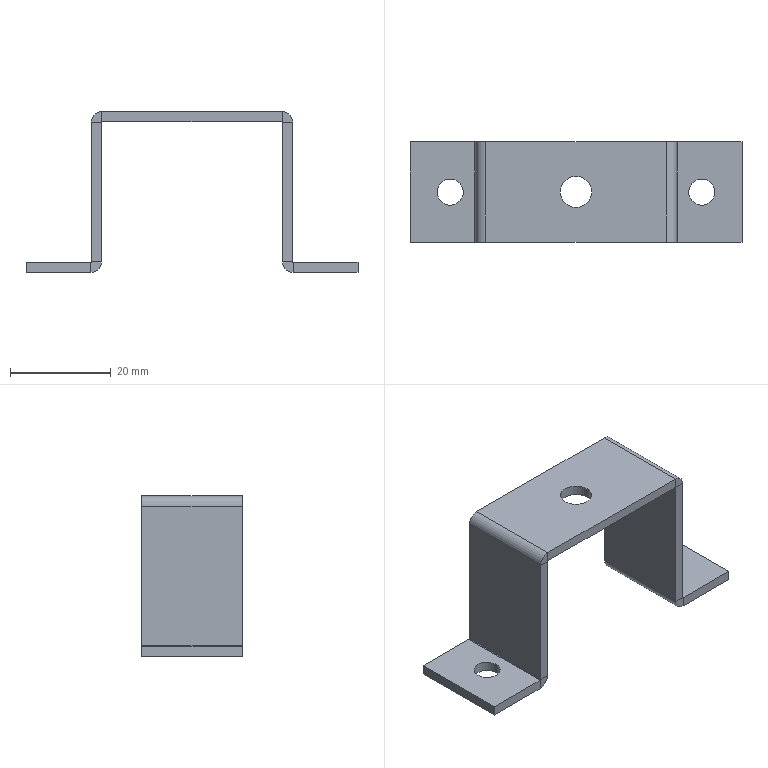Part | SolidWorks | features EdgeFlange 2, FlatPattern 1, HoleWzd 1, ICE 1, SMBaseFlange 1, SheetMetal 1 | 1 solid | 44 faces | box 66 x 20 x 32 mm | volume 4819 mm3 | plane 30 | cylinder 14 | commonest cylinder face diameters 0.2 x4 4.2 x4 5.2 x4 6.2 x2
STEP:
#1=CARTESIAN_POINT('',(-27.6,0.,-32.));
#2=VERTEX_POINT('',#1);
#3=CARTESIAN_POINT('',(-22.4,0.,-32.));
#4=VERTEX_POINT('',#3);
#5=CARTESIAN_POINT('',(-25.,0.,-32.));
#6=DIRECTION('',(0.,0.,1.));
#7=DIRECTION('',(1.,0.,0.));
#8=AXIS2_PLACEMENT_3D('',#5,#6,#7);
#9=CIRCLE('',#8,2.6);
#10=EDGE_CURVE('',#2,#4,#9,.T.);
#11=ORIENTED_EDGE('',*,*,#10,.F.);
#12=CARTESIAN_POINT('',(-27.6,0.,-30.));
#13=VERTEX_POINT('',#12);
#14=CARTESIAN_POINT('',(-27.6,0.,-30.));
#15=DIRECTION('',(0.,0.,1.));
#16=VECTOR('',#15,1000.);
#17=LINE('',#14,#16);
#18=EDGE_CURVE('',#2,#13,#17,.T.);
#19=ORIENTED_EDGE('',*,*,#18,.T.);
#20=CARTESIAN_POINT('',(-22.4,0.,-30.));
#21=VERTEX_POINT('',#20);
#22=CARTESIAN_POINT('',(-25.,0.,-30.));
#23=DIRECTION('',(0.,0.,1.));
#24=DIRECTION('',(1.,0.,0.));
#25=AXIS2_PLACEMENT_3D('',#22,#23,#24);
#26=CIRCLE('',#25,2.6);
#27=EDGE_CURVE('',#13,#21,#26,.T.);
#28=ORIENTED_EDGE('',*,*,#27,.T.);
#29=CARTESIAN_POINT('',(-22.4,0.,-30.));
#30=DIRECTION('',(0.,0.,1.));
#31=VECTOR('',#30,1000.);
#32=LINE('',#29,#31);
#33=EDGE_CURVE('',#4,#21,#32,.T.);
#34=ORIENTED_EDGE('',*,*,#33,.F.);
#35=EDGE_LOOP('',(#11,#19,#28,#34));
#36=FACE_OUTER_BOUND('',#35,.T.);
#37=CARTESIAN_POINT('',(-25.,0.,-30.));
#38=DIRECTION('',(0.,0.,1.));
#39=DIRECTION('',(1.,0.,0.));
#40=AXIS2_PLACEMENT_3D('',#37,#38,#39);
#41=CYLINDRICAL_SURFACE('',#40,2.6);
#42=ADVANCED_FACE('',(#36),#41,.F.);
#43=CARTESIAN_POINT('',(22.4,0.,-32.));
#44=VERTEX_POINT('',#43);
#45=CARTESIAN_POINT('',(27.6,0.,-32.));
#46=VERTEX_POINT('',#45);
#47=CARTESIAN_POINT('',(25.,0.,-32.));
#48=DIRECTION('',(0.,0.,1.));
#49=DIRECTION('',(1.,0.,0.));
#50=AXIS2_PLACEMENT_3D('',#47,#48,#49);
#51=CIRCLE('',#50,2.6);
#52=EDGE_CURVE('',#44,#46,#51,.T.);
#53=ORIENTED_EDGE('',*,*,#52,.F.);
#54=CARTESIAN_POINT('',(22.4,0.,-30.));
#55=VERTEX_POINT('',#54);
#56=CARTESIAN_POINT('',(22.4,0.,-30.));
#57=DIRECTION('',(0.,0.,1.));
#58=VECTOR('',#57,1000.);
#59=LINE('',#56,#58);
#60=EDGE_CURVE('',#44,#55,#59,.T.);
#61=ORIENTED_EDGE('',*,*,#60,.T.);
#62=CARTESIAN_POINT('',(27.6,0.,-30.));
#63=VERTEX_POINT('',#62);
#64=CARTESIAN_POINT('',(25.,0.,-30.));
#65=DIRECTION('',(0.,0.,1.));
#66=DIRECTION('',(1.,0.,0.));
#67=AXIS2_PLACEMENT_3D('',#64,#65,#66);
#68=CIRCLE('',#67,2.6);
#69=EDGE_CURVE('',#55,#63,#68,.T.);
#70=ORIENTED_EDGE('',*,*,#69,.T.);
#71=CARTESIAN_POINT('',(27.6,0.,-30.));
#72=DIRECTION('',(0.,0.,1.));
#73=VECTOR('',#72,1000.);
#74=LINE('',#71,#73);
#75=EDGE_CURVE('',#46,#63,#74,.T.);
#76=ORIENTED_EDGE('',*,*,#75,.F.);
#77=EDGE_LOOP('',(#53,#61,#70,#76));
#78=FACE_OUTER_BOUND('',#77,.T.);
#79=CARTESIAN_POINT('',(25.,0.,-30.));
#80=DIRECTION('',(0.,0.,1.));
#81=DIRECTION('',(1.,0.,0.));
#82=AXIS2_PLACEMENT_3D('',#79,#80,#81);
#83=CYLINDRICAL_SURFACE('',#82,2.6);
#84=ADVANCED_FACE('',(#78),#83,.F.);
#85=CARTESIAN_POINT('',(3.1,0.,-2.));
#86=VERTEX_POINT('',#85);
#87=CARTESIAN_POINT('',(-3.1,0.,-2.));
#88=VERTEX_POINT('',#87);
#89=CARTESIAN_POINT('',(0.,0.,-2.));
#90=DIRECTION('',(0.,0.,-1.));
#91=DIRECTION('',(1.,0.,0.));
#92=AXIS2_PLACEMENT_3D('',#89,#90,#91);
#93=CIRCLE('',#92,3.1);
#94=EDGE_CURVE('',#86,#88,#93,.T.);
#95=ORIENTED_EDGE('',*,*,#94,.T.);
#96=CARTESIAN_POINT('',(-3.1,0.,0.));
#97=VERTEX_POINT('',#96);
#98=CARTESIAN_POINT('',(-3.1,0.,-32.001));
#99=DIRECTION('',(0.,0.,1.));
#100=VECTOR('',#99,1000.);
#101=LINE('',#98,#100);
#102=EDGE_CURVE('',#88,#97,#101,.T.);
#103=ORIENTED_EDGE('',*,*,#102,.T.);
#104=CARTESIAN_POINT('',(3.1,0.,0.));
#105=VERTEX_POINT('',#104);
#106=CARTESIAN_POINT('',(0.,0.,0.));
#107=DIRECTION('',(0.,0.,1.));
#108=DIRECTION('',(1.,0.,0.));
#109=AXIS2_PLACEMENT_3D('',#106,#107,#108);
#110=CIRCLE('',#109,3.1);
#111=EDGE_CURVE('',#97,#105,#110,.T.);
#112=ORIENTED_EDGE('',*,*,#111,.T.);
#113=CARTESIAN_POINT('',(3.1,0.,-32.001));
#114=DIRECTION('',(0.,0.,1.));
#115=VECTOR('',#114,1000.);
#116=LINE('',#113,#115);
#117=EDGE_CURVE('',#86,#105,#116,.T.);
#118=ORIENTED_EDGE('',*,*,#117,.F.);
#119=EDGE_LOOP('',(#95,#103,#112,#118));
#120=FACE_OUTER_BOUND('',#119,.T.);
#121=CARTESIAN_POINT('',(0.,0.,-32.001));
#122=DIRECTION('',(0.,0.,1.));
#123=DIRECTION('',(1.,0.,0.));
#124=AXIS2_PLACEMENT_3D('',#121,#122,#123);
#125=CYLINDRICAL_SURFACE('',#124,3.1);
#126=ADVANCED_FACE('',(#120),#125,.F.);
#127=CARTESIAN_POINT('',(20.,10.,-2.1));
#128=VERTEX_POINT('',#127);
#129=CARTESIAN_POINT('',(20.,10.,-29.9));
#130=VERTEX_POINT('',#129);
#131=CARTESIAN_POINT('',(20.,10.,-2.));
#132=DIRECTION('',(0.,0.,-1.));
#133=VECTOR('',#132,1000.);
#134=LINE('',#131,#133);
#135=EDGE_CURVE('',#128,#130,#134,.T.);
#136=ORIENTED_EDGE('',*,*,#135,.T.);
#137=CARTESIAN_POINT('',(18.,10.,-29.9));
#138=VERTEX_POINT('',#137);
#139=CARTESIAN_POINT('',(20.,10.,-29.9));
#140=DIRECTION('',(-1.,0.,0.));
#141=VECTOR('',#140,1000.);
#142=LINE('',#139,#141);
#143=EDGE_CURVE('',#130,#138,#142,.T.);
#144=ORIENTED_EDGE('',*,*,#143,.T.);
#145=CARTESIAN_POINT('',(18.,10.,-2.1));
#146=VERTEX_POINT('',#145);
#147=CARTESIAN_POINT('',(18.,10.,0.));
#148=DIRECTION('',(0.,0.,-1.));
#149=VECTOR('',#148,1000.);
#150=LINE('',#147,#149);
#151=EDGE_CURVE('',#146,#138,#150,.T.);
#152=ORIENTED_EDGE('',*,*,#151,.F.);
#153=CARTESIAN_POINT('',(20.,10.,-2.1));
#154=DIRECTION('',(1.,0.,0.));
#155=VECTOR('',#154,1000.);
#156=LINE('',#153,#155);
#157=EDGE_CURVE('',#146,#128,#156,.T.);
#158=ORIENTED_EDGE('',*,*,#157,.T.);
#159=EDGE_LOOP('',(#136,#144,#152,#158));
#160=FACE_OUTER_BOUND('',#159,.T.);
#161=CARTESIAN_POINT('',(20.,10.,-2.));
#162=DIRECTION('',(0.,1.,0.));
#163=DIRECTION('',(0.,0.,1.));
#164=AXIS2_PLACEMENT_3D('',#161,#162,#163);
#165=PLANE('',#164);
#166=ADVANCED_FACE('',(#160),#165,.T.);
#167=CARTESIAN_POINT('',(20.,-10.,-29.9));
#168=VERTEX_POINT('',#167);
#169=CARTESIAN_POINT('',(20.,10.,-29.9));
#170=DIRECTION('',(0.,-1.,0.));
#171=VECTOR('',#170,1000.);
#172=LINE('',#169,#171);
#173=EDGE_CURVE('',#130,#168,#172,.T.);
#174=ORIENTED_EDGE('',*,*,#173,.F.);
#175=ORIENTED_EDGE('',*,*,#135,.F.);
#176=CARTESIAN_POINT('',(20.,-10.,-2.1));
#177=VERTEX_POINT('',#176);
#178=CARTESIAN_POINT('',(20.,10.,-2.1));
#179=DIRECTION('',(0.,1.,0.));
#180=VECTOR('',#179,1000.);
#181=LINE('',#178,#180);
#182=EDGE_CURVE('',#177,#128,#181,.T.);
#183=ORIENTED_EDGE('',*,*,#182,.F.);
#184=CARTESIAN_POINT('',(20.,-10.,-32.));
#185=DIRECTION('',(0.,0.,1.));
#186=VECTOR('',#185,1000.);
#187=LINE('',#184,#186);
#188=EDGE_CURVE('',#168,#177,#187,.T.);
#189=ORIENTED_EDGE('',*,*,#188,.F.);
#190=EDGE_LOOP('',(#174,#175,#183,#189));
#191=FACE_OUTER_BOUND('',#190,.T.);
#192=CARTESIAN_POINT('',(20.,0.,0.));
#193=DIRECTION('',(-1.,0.,0.));
#194=DIRECTION('',(0.,0.,1.));
#195=AXIS2_PLACEMENT_3D('',#192,#193,#194);
#196=PLANE('',#195);
#197=ADVANCED_FACE('',(#191),#196,.F.);
#198=ORIENTED_EDGE('',*,*,#151,.T.);
#199=CARTESIAN_POINT('',(18.,-10.,-29.9));
#200=VERTEX_POINT('',#199);
#201=CARTESIAN_POINT('',(18.,10.,-29.9));
#202=DIRECTION('',(0.,-1.,0.));
#203=VECTOR('',#202,1000.);
#204=LINE('',#201,#203);
#205=EDGE_CURVE('',#138,#200,#204,.T.);
#206=ORIENTED_EDGE('',*,*,#205,.T.);
#207=CARTESIAN_POINT('',(18.,-10.,-2.1));
#208=VERTEX_POINT('',#207);
#209=CARTESIAN_POINT('',(18.,-10.,0.));
#210=DIRECTION('',(0.,0.,1.));
#211=VECTOR('',#210,1000.);
#212=LINE('',#209,#211);
#213=EDGE_CURVE('',#200,#208,#212,.T.);
#214=ORIENTED_EDGE('',*,*,#213,.T.);
#215=CARTESIAN_POINT('',(18.,10.,-2.1));
#216=DIRECTION('',(0.,-1.,0.));
#217=VECTOR('',#216,1000.);
#218=LINE('',#215,#217);
#219=EDGE_CURVE('',#146,#208,#218,.T.);
#220=ORIENTED_EDGE('',*,*,#219,.F.);
#221=EDGE_LOOP('',(#198,#206,#214,#220));
#222=FACE_OUTER_BOUND('',#221,.T.);
#223=CARTESIAN_POINT('',(18.,0.,0.));
#224=DIRECTION('',(-1.,0.,0.));
#225=DIRECTION('',(0.,0.,1.));
#226=AXIS2_PLACEMENT_3D('',#223,#224,#225);
#227=PLANE('',#226);
#228=ADVANCED_FACE('',(#222),#227,.T.);
#229=CARTESIAN_POINT('',(-20.,-10.,-2.1));
#230=VERTEX_POINT('',#229);
#231=CARTESIAN_POINT('',(-20.,-10.,-29.9));
#232=VERTEX_POINT('',#231);
#233=CARTESIAN_POINT('',(-20.,-10.,-32.));
#234=DIRECTION('',(0.,0.,-1.));
#235=VECTOR('',#234,1000.);
#236=LINE('',#233,#235);
#237=EDGE_CURVE('',#230,#232,#236,.T.);
#238=ORIENTED_EDGE('',*,*,#237,.T.);
#239=CARTESIAN_POINT('',(-18.,-10.,-29.9));
#240=VERTEX_POINT('',#239);
#241=CARTESIAN_POINT('',(-20.,-10.,-29.9));
#242=DIRECTION('',(1.,0.,0.));
#243=VECTOR('',#242,1000.);
#244=LINE('',#241,#243);
#245=EDGE_CURVE('',#232,#240,#244,.T.);
#246=ORIENTED_EDGE('',*,*,#245,.T.);
#247=CARTESIAN_POINT('',(-18.,-10.,-2.1));
#248=VERTEX_POINT('',#247);
#249=CARTESIAN_POINT('',(-18.,-10.,0.));
#250=DIRECTION('',(0.,0.,-1.));
#251=VECTOR('',#250,1000.);
#252=LINE('',#249,#251);
#253=EDGE_CURVE('',#248,#240,#252,.T.);
#254=ORIENTED_EDGE('',*,*,#253,.F.);
#255=CARTESIAN_POINT('',(-20.,-10.,-2.1));
#256=DIRECTION('',(-1.,0.,0.));
#257=VECTOR('',#256,1000.);
#258=LINE('',#255,#257);
#259=EDGE_CURVE('',#248,#230,#258,.T.);
#260=ORIENTED_EDGE('',*,*,#259,.T.);
#261=EDGE_LOOP('',(#238,#246,#254,#260));
#262=FACE_OUTER_BOUND('',#261,.T.);
#263=CARTESIAN_POINT('',(-20.,-10.,-32.));
#264=DIRECTION('',(0.,-1.,0.));
#265=DIRECTION('',(0.,0.,-1.));
#266=AXIS2_PLACEMENT_3D('',#263,#264,#265);
#267=PLANE('',#266);
#268=ADVANCED_FACE('',(#262),#267,.T.);
#269=CARTESIAN_POINT('',(-20.,10.,-29.9));
#270=VERTEX_POINT('',#269);
#271=CARTESIAN_POINT('',(-20.,10.,-2.1));
#272=VERTEX_POINT('',#271);
#273=CARTESIAN_POINT('',(-20.,10.,-2.));
#274=DIRECTION('',(0.,0.,1.));
#275=VECTOR('',#274,1000.);
#276=LINE('',#273,#275);
#277=EDGE_CURVE('',#270,#272,#276,.T.);
#278=ORIENTED_EDGE('',*,*,#277,.F.);
#279=CARTESIAN_POINT('',(-20.,-10.,-29.9));
#280=DIRECTION('',(0.,1.,0.));
#281=VECTOR('',#280,1000.);
#282=LINE('',#279,#281);
#283=EDGE_CURVE('',#232,#270,#282,.T.);
#284=ORIENTED_EDGE('',*,*,#283,.F.);
#285=ORIENTED_EDGE('',*,*,#237,.F.);
#286=CARTESIAN_POINT('',(-20.,0.,-2.1));
#287=DIRECTION('',(0.,1.,0.));
#288=VECTOR('',#287,1000.);
#289=LINE('',#286,#288);
#290=EDGE_CURVE('',#230,#272,#289,.T.);
#291=ORIENTED_EDGE('',*,*,#290,.T.);
#292=EDGE_LOOP('',(#278,#284,#285,#291));
#293=FACE_OUTER_BOUND('',#292,.T.);
#294=CARTESIAN_POINT('',(-20.,0.,0.));
#295=DIRECTION('',(-1.,0.,0.));
#296=DIRECTION('',(0.,0.,1.));
#297=AXIS2_PLACEMENT_3D('',#294,#295,#296);
#298=PLANE('',#297);
#299=ADVANCED_FACE('',(#293),#298,.T.);
#300=CARTESIAN_POINT('',(-18.,10.,-29.9));
#301=VERTEX_POINT('',#300);
#302=CARTESIAN_POINT('',(-18.,-10.,-29.9));
#303=DIRECTION('',(0.,1.,0.));
#304=VECTOR('',#303,1000.);
#305=LINE('',#302,#304);
#306=EDGE_CURVE('',#240,#301,#305,.T.);
#307=ORIENTED_EDGE('',*,*,#306,.T.);
#308=CARTESIAN_POINT('',(-18.,10.,-2.1));
#309=VERTEX_POINT('',#308);
#310=CARTESIAN_POINT('',(-18.,10.,0.));
#311=DIRECTION('',(0.,0.,1.));
#312=VECTOR('',#311,1000.);
#313=LINE('',#310,#312);
#314=EDGE_CURVE('',#301,#309,#313,.T.);
#315=ORIENTED_EDGE('',*,*,#314,.T.);
#316=CARTESIAN_POINT('',(-18.,-10.,-2.1));
#317=DIRECTION('',(0.,1.,0.));
#318=VECTOR('',#317,1000.);
#319=LINE('',#316,#318);
#320=EDGE_CURVE('',#248,#309,#319,.T.);
#321=ORIENTED_EDGE('',*,*,#320,.F.);
#322=ORIENTED_EDGE('',*,*,#253,.T.);
#323=EDGE_LOOP('',(#307,#315,#321,#322));
#324=FACE_OUTER_BOUND('',#323,.T.);
#325=CARTESIAN_POINT('',(-18.,0.,0.));
#326=DIRECTION('',(-1.,0.,0.));
#327=DIRECTION('',(0.,0.,1.));
#328=AXIS2_PLACEMENT_3D('',#325,#326,#327);
#329=PLANE('',#328);
#330=ADVANCED_FACE('',(#324),#329,.F.);
#331=ORIENTED_EDGE('',*,*,#94,.F.);
#332=CARTESIAN_POINT('',(0.,0.,-2.));
#333=DIRECTION('',(0.,0.,-1.));
#334=DIRECTION('',(1.,0.,0.));
#335=AXIS2_PLACEMENT_3D('',#332,#333,#334);
#336=CIRCLE('',#335,3.1);
#337=EDGE_CURVE('',#88,#86,#336,.T.);
#338=ORIENTED_EDGE('',*,*,#337,.F.);
#339=EDGE_LOOP('',(#331,#338));
#340=FACE_BOUND('',#339,.T.);
#341=CARTESIAN_POINT('',(17.9,-10.,-2.));
#342=VERTEX_POINT('',#341);
#343=CARTESIAN_POINT('',(17.9,10.,-2.));
#344=VERTEX_POINT('',#343);
#345=CARTESIAN_POINT('',(17.9,-10.,-2.));
#346=DIRECTION('',(0.,1.,0.));
#347=VECTOR('',#346,1000.);
#348=LINE('',#345,#347);
#349=EDGE_CURVE('',#342,#344,#348,.T.);
#350=ORIENTED_EDGE('',*,*,#349,.F.);
#351=CARTESIAN_POINT('',(-17.9,-10.,-2.));
#352=VERTEX_POINT('',#351);
#353=CARTESIAN_POINT('',(-20.,-10.,-2.));
#354=DIRECTION('',(1.,0.,0.));
#355=VECTOR('',#354,1000.);
#356=LINE('',#353,#355);
#357=EDGE_CURVE('',#352,#342,#356,.T.);
#358=ORIENTED_EDGE('',*,*,#357,.F.);
#359=CARTESIAN_POINT('',(-17.9,10.,-2.));
#360=VERTEX_POINT('',#359);
#361=CARTESIAN_POINT('',(-17.9,10.,-2.));
#362=DIRECTION('',(0.,-1.,0.));
#363=VECTOR('',#362,1000.);
#364=LINE('',#361,#363);
#365=EDGE_CURVE('',#360,#352,#364,.T.);
#366=ORIENTED_EDGE('',*,*,#365,.F.);
#367=CARTESIAN_POINT('',(-20.,10.,-2.));
#368=DIRECTION('',(-1.,0.,0.));
#369=VECTOR('',#368,1000.);
#370=LINE('',#367,#369);
#371=EDGE_CURVE('',#344,#360,#370,.T.);
#372=ORIENTED_EDGE('',*,*,#371,.F.);
#373=EDGE_LOOP('',(#350,#358,#366,#372));
#374=FACE_OUTER_BOUND('',#373,.T.);
#375=CARTESIAN_POINT('',(0.,0.,-2.));
#376=DIRECTION('',(0.,0.,1.));
#377=DIRECTION('',(1.,0.,0.));
#378=AXIS2_PLACEMENT_3D('',#375,#376,#377);
#379=PLANE('',#378);
#380=ADVANCED_FACE('',(#340,#374),#379,.F.);
#381=CARTESIAN_POINT('',(0.,0.,0.));
#382=DIRECTION('',(0.,0.,1.));
#383=DIRECTION('',(1.,0.,0.));
#384=AXIS2_PLACEMENT_3D('',#381,#382,#383);
#385=CIRCLE('',#384,3.1);
#386=EDGE_CURVE('',#105,#97,#385,.T.);
#387=ORIENTED_EDGE('',*,*,#386,.F.);
#388=ORIENTED_EDGE('',*,*,#111,.F.);
#389=EDGE_LOOP('',(#387,#388));
#390=FACE_BOUND('',#389,.T.);
#391=CARTESIAN_POINT('',(-17.9,-10.,0.));
#392=VERTEX_POINT('',#391);
#393=CARTESIAN_POINT('',(17.9,-10.,0.));
#394=VERTEX_POINT('',#393);
#395=CARTESIAN_POINT('',(-20.,-10.,0.));
#396=DIRECTION('',(1.,0.,0.));
#397=VECTOR('',#396,1000.);
#398=LINE('',#395,#397);
#399=EDGE_CURVE('',#392,#394,#398,.T.);
#400=ORIENTED_EDGE('',*,*,#399,.T.);
#401=CARTESIAN_POINT('',(17.9,10.,0.));
#402=VERTEX_POINT('',#401);
#403=CARTESIAN_POINT('',(17.9,-10.,0.));
#404=DIRECTION('',(0.,1.,0.));
#405=VECTOR('',#404,1000.);
#406=LINE('',#403,#405);
#407=EDGE_CURVE('',#394,#402,#406,.T.);
#408=ORIENTED_EDGE('',*,*,#407,.T.);
#409=CARTESIAN_POINT('',(-17.9,10.,0.));
#410=VERTEX_POINT('',#409);
#411=CARTESIAN_POINT('',(-20.,10.,0.));
#412=DIRECTION('',(-1.,0.,0.));
#413=VECTOR('',#412,1000.);
#414=LINE('',#411,#413);
#415=EDGE_CURVE('',#402,#410,#414,.T.);
#416=ORIENTED_EDGE('',*,*,#415,.T.);
#417=CARTESIAN_POINT('',(-17.9,10.,0.));
#418=DIRECTION('',(0.,-1.,0.));
#419=VECTOR('',#418,1000.);
#420=LINE('',#417,#419);
#421=EDGE_CURVE('',#410,#392,#420,.T.);
#422=ORIENTED_EDGE('',*,*,#421,.T.);
#423=EDGE_LOOP('',(#400,#408,#416,#422));
#424=FACE_OUTER_BOUND('',#423,.T.);
#425=CARTESIAN_POINT('',(0.,0.,0.));
#426=DIRECTION('',(0.,0.,1.));
#427=DIRECTION('',(1.,0.,0.));
#428=AXIS2_PLACEMENT_3D('',#425,#426,#427);
#429=PLANE('',#428);
#430=ADVANCED_FACE('',(#390,#424),#429,.T.);
#431=ORIENTED_EDGE('',*,*,#357,.T.);
#432=CARTESIAN_POINT('',(17.9,-10.,-2.));
#433=DIRECTION('',(0.,0.,1.));
#434=VECTOR('',#433,1000.);
#435=LINE('',#432,#434);
#436=EDGE_CURVE('',#342,#394,#435,.T.);
#437=ORIENTED_EDGE('',*,*,#436,.T.);
#438=ORIENTED_EDGE('',*,*,#399,.F.);
#439=CARTESIAN_POINT('',(-17.9,-10.,-2.));
#440=DIRECTION('',(0.,0.,1.));
#441=VECTOR('',#440,1000.);
#442=LINE('',#439,#441);
#443=EDGE_CURVE('',#352,#392,#442,.T.);
#444=ORIENTED_EDGE('',*,*,#443,.F.);
#445=EDGE_LOOP('',(#431,#437,#438,#444));
#446=FACE_OUTER_BOUND('',#445,.T.);
#447=CARTESIAN_POINT('',(-20.,-10.,-2.));
#448=DIRECTION('',(0.,-1.,0.));
#449=DIRECTION('',(0.,0.,-1.));
#450=AXIS2_PLACEMENT_3D('',#447,#448,#449);
#451=PLANE('',#450);
#452=ADVANCED_FACE('',(#446),#451,.T.);
#453=CARTESIAN_POINT('',(17.9,10.,-2.));
#454=DIRECTION('',(0.,0.,1.));
#455=VECTOR('',#454,1000.);
#456=LINE('',#453,#455);
#457=EDGE_CURVE('',#344,#402,#456,.T.);
#458=ORIENTED_EDGE('',*,*,#457,.F.);
#459=ORIENTED_EDGE('',*,*,#371,.T.);
#460=CARTESIAN_POINT('',(-17.9,10.,-2.));
#461=DIRECTION('',(0.,0.,1.));
#462=VECTOR('',#461,1000.);
#463=LINE('',#460,#462);
#464=EDGE_CURVE('',#360,#410,#463,.T.);
#465=ORIENTED_EDGE('',*,*,#464,.T.);
#466=ORIENTED_EDGE('',*,*,#415,.F.);
#467=EDGE_LOOP('',(#458,#459,#465,#466));
#468=FACE_OUTER_BOUND('',#467,.T.);
#469=CARTESIAN_POINT('',(-20.,10.,-2.));
#470=DIRECTION('',(0.,1.,0.));
#471=DIRECTION('',(0.,0.,1.));
#472=AXIS2_PLACEMENT_3D('',#469,#470,#471);
#473=PLANE('',#472);
#474=ADVANCED_FACE('',(#468),#473,.T.);
#475=ORIENTED_EDGE('',*,*,#259,.F.);
#476=CARTESIAN_POINT('',(-17.9,-10.,-2.1));
#477=DIRECTION('',(0.,-1.,0.));
#478=DIRECTION('',(0.,0.,1.));
#479=AXIS2_PLACEMENT_3D('',#476,#477,#478);
#480=CIRCLE('',#479,0.1);
#481=EDGE_CURVE('',#352,#248,#480,.T.);
#482=ORIENTED_EDGE('',*,*,#481,.F.);
#483=ORIENTED_EDGE('',*,*,#443,.T.);
#484=CARTESIAN_POINT('',(-17.9,-10.,-2.1));
#485=DIRECTION('',(0.,-1.,0.));
#486=DIRECTION('',(0.,0.,1.));
#487=AXIS2_PLACEMENT_3D('',#484,#485,#486);
#488=CIRCLE('',#487,2.1);
#489=EDGE_CURVE('',#392,#230,#488,.T.);
#490=ORIENTED_EDGE('',*,*,#489,.T.);
#491=EDGE_LOOP('',(#475,#482,#483,#490));
#492=FACE_OUTER_BOUND('',#491,.T.);
#493=CARTESIAN_POINT('',(-17.9,-10.,-2.1));
#494=DIRECTION('',(0.,-1.,0.));
#495=DIRECTION('',(0.,0.,-1.));
#496=AXIS2_PLACEMENT_3D('',#493,#494,#495);
#497=PLANE('',#496);
#498=ADVANCED_FACE('',(#492),#497,.T.);
#499=CARTESIAN_POINT('',(-17.9,10.,-2.1));
#500=DIRECTION('',(0.,1.,0.));
#501=DIRECTION('',(0.,0.,1.));
#502=AXIS2_PLACEMENT_3D('',#499,#500,#501);
#503=CIRCLE('',#502,0.1);
#504=EDGE_CURVE('',#309,#360,#503,.T.);
#505=ORIENTED_EDGE('',*,*,#504,.F.);
#506=CARTESIAN_POINT('',(-18.,10.,-2.1));
#507=DIRECTION('',(-1.,0.,0.));
#508=VECTOR('',#507,1000.);
#509=LINE('',#506,#508);
#510=EDGE_CURVE('',#309,#272,#509,.T.);
#511=ORIENTED_EDGE('',*,*,#510,.T.);
#512=CARTESIAN_POINT('',(-17.9,10.,-2.1));
#513=DIRECTION('',(0.,1.,0.));
#514=DIRECTION('',(0.,0.,1.));
#515=AXIS2_PLACEMENT_3D('',#512,#513,#514);
#516=CIRCLE('',#515,2.1);
#517=EDGE_CURVE('',#272,#410,#516,.T.);
#518=ORIENTED_EDGE('',*,*,#517,.T.);
#519=ORIENTED_EDGE('',*,*,#464,.F.);
#520=EDGE_LOOP('',(#505,#511,#518,#519));
#521=FACE_OUTER_BOUND('',#520,.T.);
#522=CARTESIAN_POINT('',(-17.9,10.,-2.1));
#523=DIRECTION('',(0.,-1.,0.));
#524=DIRECTION('',(0.,0.,-1.));
#525=AXIS2_PLACEMENT_3D('',#522,#523,#524);
#526=PLANE('',#525);
#527=ADVANCED_FACE('',(#521),#526,.F.);
#528=ORIENTED_EDGE('',*,*,#421,.F.);
#529=ORIENTED_EDGE('',*,*,#517,.F.);
#530=ORIENTED_EDGE('',*,*,#290,.F.);
#531=ORIENTED_EDGE('',*,*,#489,.F.);
#532=EDGE_LOOP('',(#528,#529,#530,#531));
#533=FACE_OUTER_BOUND('',#532,.T.);
#534=CARTESIAN_POINT('',(-17.9,10.,-2.1));
#535=DIRECTION('',(0.,1.,0.));
#536=DIRECTION('',(-1.,0.,0.));
#537=AXIS2_PLACEMENT_3D('',#534,#535,#536);
#538=CYLINDRICAL_SURFACE('',#537,2.1);
#539=ADVANCED_FACE('',(#533),#538,.T.);
#540=ORIENTED_EDGE('',*,*,#365,.T.);
#541=ORIENTED_EDGE('',*,*,#481,.T.);
#542=ORIENTED_EDGE('',*,*,#320,.T.);
#543=ORIENTED_EDGE('',*,*,#504,.T.);
#544=EDGE_LOOP('',(#540,#541,#542,#543));
#545=FACE_OUTER_BOUND('',#544,.T.);
#546=CARTESIAN_POINT('',(-17.9,10.,-2.1));
#547=DIRECTION('',(0.,1.,0.));
#548=DIRECTION('',(-1.,0.,0.));
#549=AXIS2_PLACEMENT_3D('',#546,#547,#548);
#550=CYLINDRICAL_SURFACE('',#549,0.1);
#551=ADVANCED_FACE('',(#545),#550,.F.);
#552=CARTESIAN_POINT('',(-20.,10.,-29.9));
#553=DIRECTION('',(1.,0.,0.));
#554=VECTOR('',#553,1000.);
#555=LINE('',#552,#554);
#556=EDGE_CURVE('',#270,#301,#555,.T.);
#557=ORIENTED_EDGE('',*,*,#556,.F.);
#558=ORIENTED_EDGE('',*,*,#277,.T.);
#559=ORIENTED_EDGE('',*,*,#510,.F.);
#560=ORIENTED_EDGE('',*,*,#314,.F.);
#561=EDGE_LOOP('',(#557,#558,#559,#560));
#562=FACE_OUTER_BOUND('',#561,.T.);
#563=CARTESIAN_POINT('',(-20.,10.,-2.));
#564=DIRECTION('',(0.,1.,0.));
#565=DIRECTION('',(0.,0.,1.));
#566=AXIS2_PLACEMENT_3D('',#563,#564,#565);
#567=PLANE('',#566);
#568=ADVANCED_FACE('',(#562),#567,.T.);
#569=ORIENTED_EDGE('',*,*,#157,.F.);
#570=CARTESIAN_POINT('',(17.9,10.,-2.1));
#571=DIRECTION('',(0.,1.,0.));
#572=DIRECTION('',(0.,0.,-1.));
#573=AXIS2_PLACEMENT_3D('',#570,#571,#572);
#574=CIRCLE('',#573,0.1);
#575=EDGE_CURVE('',#344,#146,#574,.T.);
#576=ORIENTED_EDGE('',*,*,#575,.F.);
#577=ORIENTED_EDGE('',*,*,#457,.T.);
#578=CARTESIAN_POINT('',(17.9,10.,-2.1));
#579=DIRECTION('',(0.,1.,0.));
#580=DIRECTION('',(0.,0.,-1.));
#581=AXIS2_PLACEMENT_3D('',#578,#579,#580);
#582=CIRCLE('',#581,2.1);
#583=EDGE_CURVE('',#402,#128,#582,.T.);
#584=ORIENTED_EDGE('',*,*,#583,.T.);
#585=EDGE_LOOP('',(#569,#576,#577,#584));
#586=FACE_OUTER_BOUND('',#585,.T.);
#587=CARTESIAN_POINT('',(17.9,10.,-2.1));
#588=DIRECTION('',(0.,1.,0.));
#589=DIRECTION('',(0.,0.,1.));
#590=AXIS2_PLACEMENT_3D('',#587,#588,#589);
#591=PLANE('',#590);
#592=ADVANCED_FACE('',(#586),#591,.T.);
#593=CARTESIAN_POINT('',(17.9,-10.,-2.1));
#594=DIRECTION('',(0.,-1.,0.));
#595=DIRECTION('',(0.,0.,-1.));
#596=AXIS2_PLACEMENT_3D('',#593,#594,#595);
#597=CIRCLE('',#596,0.1);
#598=EDGE_CURVE('',#208,#342,#597,.T.);
#599=ORIENTED_EDGE('',*,*,#598,.F.);
#600=CARTESIAN_POINT('',(18.,-10.,-2.1));
#601=DIRECTION('',(1.,0.,0.));
#602=VECTOR('',#601,1000.);
#603=LINE('',#600,#602);
#604=EDGE_CURVE('',#208,#177,#603,.T.);
#605=ORIENTED_EDGE('',*,*,#604,.T.);
#606=CARTESIAN_POINT('',(17.9,-10.,-2.1));
#607=DIRECTION('',(0.,-1.,0.));
#608=DIRECTION('',(0.,0.,-1.));
#609=AXIS2_PLACEMENT_3D('',#606,#607,#608);
#610=CIRCLE('',#609,2.1);
#611=EDGE_CURVE('',#177,#394,#610,.T.);
#612=ORIENTED_EDGE('',*,*,#611,.T.);
#613=ORIENTED_EDGE('',*,*,#436,.F.);
#614=EDGE_LOOP('',(#599,#605,#612,#613));
#615=FACE_OUTER_BOUND('',#614,.T.);
#616=CARTESIAN_POINT('',(17.9,-10.,-2.1));
#617=DIRECTION('',(0.,1.,0.));
#618=DIRECTION('',(0.,0.,1.));
#619=AXIS2_PLACEMENT_3D('',#616,#617,#618);
#620=PLANE('',#619);
#621=ADVANCED_FACE('',(#615),#620,.F.);
#622=ORIENTED_EDGE('',*,*,#407,.F.);
#623=ORIENTED_EDGE('',*,*,#611,.F.);
#624=ORIENTED_EDGE('',*,*,#182,.T.);
#625=ORIENTED_EDGE('',*,*,#583,.F.);
#626=EDGE_LOOP('',(#622,#623,#624,#625));
#627=FACE_OUTER_BOUND('',#626,.T.);
#628=CARTESIAN_POINT('',(17.9,-10.,-2.1));
#629=DIRECTION('',(0.,-1.,0.));
#630=DIRECTION('',(1.,0.,0.));
#631=AXIS2_PLACEMENT_3D('',#628,#629,#630);
#632=CYLINDRICAL_SURFACE('',#631,2.1);
#633=ADVANCED_FACE('',(#627),#632,.T.);
#634=ORIENTED_EDGE('',*,*,#349,.T.);
#635=ORIENTED_EDGE('',*,*,#575,.T.);
#636=ORIENTED_EDGE('',*,*,#219,.T.);
#637=ORIENTED_EDGE('',*,*,#598,.T.);
#638=EDGE_LOOP('',(#634,#635,#636,#637));
#639=FACE_OUTER_BOUND('',#638,.T.);
#640=CARTESIAN_POINT('',(17.9,-10.,-2.1));
#641=DIRECTION('',(0.,-1.,0.));
#642=DIRECTION('',(1.,0.,0.));
#643=AXIS2_PLACEMENT_3D('',#640,#641,#642);
#644=CYLINDRICAL_SURFACE('',#643,0.1);
#645=ADVANCED_FACE('',(#639),#644,.F.);
#646=CARTESIAN_POINT('',(20.,-10.,-29.9));
#647=DIRECTION('',(-1.,0.,0.));
#648=VECTOR('',#647,1000.);
#649=LINE('',#646,#648);
#650=EDGE_CURVE('',#168,#200,#649,.T.);
#651=ORIENTED_EDGE('',*,*,#650,.F.);
#652=ORIENTED_EDGE('',*,*,#188,.T.);
#653=ORIENTED_EDGE('',*,*,#604,.F.);
#654=ORIENTED_EDGE('',*,*,#213,.F.);
#655=EDGE_LOOP('',(#651,#652,#653,#654));
#656=FACE_OUTER_BOUND('',#655,.T.);
#657=CARTESIAN_POINT('',(20.,-10.,-32.));
#658=DIRECTION('',(0.,-1.,0.));
#659=DIRECTION('',(0.,0.,-1.));
#660=AXIS2_PLACEMENT_3D('',#657,#658,#659);
#661=PLANE('',#660);
#662=ADVANCED_FACE('',(#656),#661,.T.);
#663=CARTESIAN_POINT('',(-20.1,10.,-30.));
#664=VERTEX_POINT('',#663);
#665=CARTESIAN_POINT('',(-20.1,10.,-32.));
#666=VERTEX_POINT('',#665);
#667=CARTESIAN_POINT('',(-20.1,10.,-32.));
#668=DIRECTION('',(0.,0.,-1.));
#669=VECTOR('',#668,1000.);
#670=LINE('',#667,#669);
#671=EDGE_CURVE('',#664,#666,#670,.T.);
#672=ORIENTED_EDGE('',*,*,#671,.F.);
#673=CARTESIAN_POINT('',(-20.1,10.,-29.9));
#674=DIRECTION('',(0.,1.,0.));
#675=DIRECTION('',(0.,0.,-1.));
#676=AXIS2_PLACEMENT_3D('',#673,#674,#675);
#677=CIRCLE('',#676,0.1);
#678=EDGE_CURVE('',#270,#664,#677,.T.);
#679=ORIENTED_EDGE('',*,*,#678,.F.);
#680=ORIENTED_EDGE('',*,*,#556,.T.);
#681=CARTESIAN_POINT('',(-20.1,10.,-29.9));
#682=DIRECTION('',(0.,1.,0.));
#683=DIRECTION('',(0.,0.,-1.));
#684=AXIS2_PLACEMENT_3D('',#681,#682,#683);
#685=CIRCLE('',#684,2.1);
#686=EDGE_CURVE('',#301,#666,#685,.T.);
#687=ORIENTED_EDGE('',*,*,#686,.T.);
#688=EDGE_LOOP('',(#672,#679,#680,#687));
#689=FACE_OUTER_BOUND('',#688,.T.);
#690=CARTESIAN_POINT('',(-20.1,10.,-29.9));
#691=DIRECTION('',(0.,1.,0.));
#692=DIRECTION('',(0.,0.,1.));
#693=AXIS2_PLACEMENT_3D('',#690,#691,#692);
#694=PLANE('',#693);
#695=ADVANCED_FACE('',(#689),#694,.T.);
#696=CARTESIAN_POINT('',(-20.1,-10.,-30.));
#697=VERTEX_POINT('',#696);
#698=CARTESIAN_POINT('',(-20.1,-10.,-29.9));
#699=DIRECTION('',(0.,-1.,0.));
#700=DIRECTION('',(0.,0.,-1.));
#701=AXIS2_PLACEMENT_3D('',#698,#699,#700);
#702=CIRCLE('',#701,0.1);
#703=EDGE_CURVE('',#697,#232,#702,.T.);
#704=ORIENTED_EDGE('',*,*,#703,.F.);
#705=CARTESIAN_POINT('',(-20.1,-10.,-32.));
#706=VERTEX_POINT('',#705);
#707=CARTESIAN_POINT('',(-20.1,-10.,-30.));
#708=DIRECTION('',(0.,0.,-1.));
#709=VECTOR('',#708,1000.);
#710=LINE('',#707,#709);
#711=EDGE_CURVE('',#697,#706,#710,.T.);
#712=ORIENTED_EDGE('',*,*,#711,.T.);
#713=CARTESIAN_POINT('',(-20.1,-10.,-29.9));
#714=DIRECTION('',(0.,-1.,0.));
#715=DIRECTION('',(0.,0.,-1.));
#716=AXIS2_PLACEMENT_3D('',#713,#714,#715);
#717=CIRCLE('',#716,2.1);
#718=EDGE_CURVE('',#706,#240,#717,.T.);
#719=ORIENTED_EDGE('',*,*,#718,.T.);
#720=ORIENTED_EDGE('',*,*,#245,.F.);
#721=EDGE_LOOP('',(#704,#712,#719,#720));
#722=FACE_OUTER_BOUND('',#721,.T.);
#723=CARTESIAN_POINT('',(-20.1,-10.,-29.9));
#724=DIRECTION('',(0.,1.,0.));
#725=DIRECTION('',(0.,0.,1.));
#726=AXIS2_PLACEMENT_3D('',#723,#724,#725);
#727=PLANE('',#726);
#728=ADVANCED_FACE('',(#722),#727,.F.);
#729=ORIENTED_EDGE('',*,*,#306,.F.);
#730=ORIENTED_EDGE('',*,*,#718,.F.);
#731=CARTESIAN_POINT('',(-20.1,10.,-32.));
#732=DIRECTION('',(0.,1.,0.));
#733=VECTOR('',#732,1000.);
#734=LINE('',#731,#733);
#735=EDGE_CURVE('',#706,#666,#734,.T.);
#736=ORIENTED_EDGE('',*,*,#735,.T.);
#737=ORIENTED_EDGE('',*,*,#686,.F.);
#738=EDGE_LOOP('',(#729,#730,#736,#737));
#739=FACE_OUTER_BOUND('',#738,.T.);
#740=CARTESIAN_POINT('',(-20.1,-10.,-29.9));
#741=DIRECTION('',(0.,-1.,0.));
#742=DIRECTION('',(0.,0.,-1.));
#743=AXIS2_PLACEMENT_3D('',#740,#741,#742);
#744=CYLINDRICAL_SURFACE('',#743,2.1);
#745=ADVANCED_FACE('',(#739),#744,.T.);
#746=ORIENTED_EDGE('',*,*,#283,.T.);
#747=ORIENTED_EDGE('',*,*,#678,.T.);
#748=CARTESIAN_POINT('',(-20.1,10.,-30.));
#749=DIRECTION('',(0.,-1.,0.));
#750=VECTOR('',#749,1000.);
#751=LINE('',#748,#750);
#752=EDGE_CURVE('',#664,#697,#751,.T.);
#753=ORIENTED_EDGE('',*,*,#752,.T.);
#754=ORIENTED_EDGE('',*,*,#703,.T.);
#755=EDGE_LOOP('',(#746,#747,#753,#754));
#756=FACE_OUTER_BOUND('',#755,.T.);
#757=CARTESIAN_POINT('',(-20.1,-10.,-29.9));
#758=DIRECTION('',(0.,-1.,0.));
#759=DIRECTION('',(0.,0.,-1.));
#760=AXIS2_PLACEMENT_3D('',#757,#758,#759);
#761=CYLINDRICAL_SURFACE('',#760,0.1);
#762=ADVANCED_FACE('',(#756),#761,.F.);
#763=ORIENTED_EDGE('',*,*,#711,.F.);
#764=CARTESIAN_POINT('',(-33.,-10.,-30.));
#765=VERTEX_POINT('',#764);
#766=CARTESIAN_POINT('',(-33.,-10.,-30.));
#767=DIRECTION('',(-1.,0.,0.));
#768=VECTOR('',#767,1000.);
#769=LINE('',#766,#768);
#770=EDGE_CURVE('',#697,#765,#769,.T.);
#771=ORIENTED_EDGE('',*,*,#770,.T.);
#772=CARTESIAN_POINT('',(-33.,-10.,-32.));
#773=VERTEX_POINT('',#772);
#774=CARTESIAN_POINT('',(-33.,-10.,-32.));
#775=DIRECTION('',(0.,0.,1.));
#776=VECTOR('',#775,1000.);
#777=LINE('',#774,#776);
#778=EDGE_CURVE('',#773,#765,#777,.T.);
#779=ORIENTED_EDGE('',*,*,#778,.F.);
#780=CARTESIAN_POINT('',(0.,-10.,-32.));
#781=DIRECTION('',(-1.,0.,0.));
#782=VECTOR('',#781,1000.);
#783=LINE('',#780,#782);
#784=EDGE_CURVE('',#706,#773,#783,.T.);
#785=ORIENTED_EDGE('',*,*,#784,.F.);
#786=EDGE_LOOP('',(#763,#771,#779,#785));
#787=FACE_OUTER_BOUND('',#786,.T.);
#788=CARTESIAN_POINT('',(-33.,-10.,-32.));
#789=DIRECTION('',(0.,1.,0.));
#790=DIRECTION('',(-1.,0.,0.));
#791=AXIS2_PLACEMENT_3D('',#788,#789,#790);
#792=PLANE('',#791);
#793=ADVANCED_FACE('',(#787),#792,.F.);
#794=ORIENTED_EDGE('',*,*,#671,.T.);
#795=CARTESIAN_POINT('',(-33.,10.,-32.));
#796=VERTEX_POINT('',#795);
#797=CARTESIAN_POINT('',(0.,10.,-32.));
#798=DIRECTION('',(1.,0.,0.));
#799=VECTOR('',#798,1000.);
#800=LINE('',#797,#799);
#801=EDGE_CURVE('',#796,#666,#800,.T.);
#802=ORIENTED_EDGE('',*,*,#801,.F.);
#803=CARTESIAN_POINT('',(-33.,10.,-30.));
#804=VERTEX_POINT('',#803);
#805=CARTESIAN_POINT('',(-33.,10.,-32.));
#806=DIRECTION('',(0.,0.,1.));
#807=VECTOR('',#806,1000.);
#808=LINE('',#805,#807);
#809=EDGE_CURVE('',#796,#804,#808,.T.);
#810=ORIENTED_EDGE('',*,*,#809,.T.);
#811=CARTESIAN_POINT('',(-20.,10.,-30.));
#812=DIRECTION('',(1.,0.,0.));
#813=VECTOR('',#812,1000.);
#814=LINE('',#811,#813);
#815=EDGE_CURVE('',#804,#664,#814,.T.);
#816=ORIENTED_EDGE('',*,*,#815,.T.);
#817=EDGE_LOOP('',(#794,#802,#810,#816));
#818=FACE_OUTER_BOUND('',#817,.T.);
#819=CARTESIAN_POINT('',(-20.,10.,-32.));
#820=DIRECTION('',(0.,-1.,0.));
#821=DIRECTION('',(0.,0.,-1.));
#822=AXIS2_PLACEMENT_3D('',#819,#820,#821);
#823=PLANE('',#822);
#824=ADVANCED_FACE('',(#818),#823,.F.);
#825=CARTESIAN_POINT('',(-25.,0.,-32.));
#826=DIRECTION('',(0.,0.,1.));
#827=DIRECTION('',(1.,0.,0.));
#828=AXIS2_PLACEMENT_3D('',#825,#826,#827);
#829=CIRCLE('',#828,2.6);
#830=EDGE_CURVE('',#4,#2,#829,.T.);
#831=ORIENTED_EDGE('',*,*,#830,.T.);
#832=ORIENTED_EDGE('',*,*,#10,.T.);
#833=EDGE_LOOP('',(#831,#832));
#834=FACE_BOUND('',#833,.T.);
#835=ORIENTED_EDGE('',*,*,#735,.F.);
#836=ORIENTED_EDGE('',*,*,#784,.T.);
#837=CARTESIAN_POINT('',(-33.,0.,-32.));
#838=DIRECTION('',(0.,1.,0.));
#839=VECTOR('',#838,1000.);
#840=LINE('',#837,#839);
#841=EDGE_CURVE('',#773,#796,#840,.T.);
#842=ORIENTED_EDGE('',*,*,#841,.T.);
#843=ORIENTED_EDGE('',*,*,#801,.T.);
#844=EDGE_LOOP('',(#835,#836,#842,#843));
#845=FACE_OUTER_BOUND('',#844,.T.);
#846=CARTESIAN_POINT('',(0.,0.,-32.));
#847=DIRECTION('',(0.,0.,1.));
#848=DIRECTION('',(1.,0.,0.));
#849=AXIS2_PLACEMENT_3D('',#846,#847,#848);
#850=PLANE('',#849);
#851=ADVANCED_FACE('',(#834,#845),#850,.F.);
#852=CARTESIAN_POINT('',(-25.,0.,-30.));
#853=DIRECTION('',(0.,0.,1.));
#854=DIRECTION('',(1.,0.,0.));
#855=AXIS2_PLACEMENT_3D('',#852,#853,#854);
#856=CIRCLE('',#855,2.6);
#857=EDGE_CURVE('',#21,#13,#856,.T.);
#858=ORIENTED_EDGE('',*,*,#857,.F.);
#859=ORIENTED_EDGE('',*,*,#27,.F.);
#860=EDGE_LOOP('',(#858,#859));
#861=FACE_BOUND('',#860,.T.);
#862=ORIENTED_EDGE('',*,*,#770,.F.);
#863=ORIENTED_EDGE('',*,*,#752,.F.);
#864=ORIENTED_EDGE('',*,*,#815,.F.);
#865=CARTESIAN_POINT('',(-33.,10.,-30.));
#866=DIRECTION('',(0.,1.,0.));
#867=VECTOR('',#866,1000.);
#868=LINE('',#865,#867);
#869=EDGE_CURVE('',#765,#804,#868,.T.);
#870=ORIENTED_EDGE('',*,*,#869,.F.);
#871=EDGE_LOOP('',(#862,#863,#864,#870));
#872=FACE_OUTER_BOUND('',#871,.T.);
#873=CARTESIAN_POINT('',(0.,0.,-30.));
#874=DIRECTION('',(0.,0.,1.));
#875=DIRECTION('',(1.,0.,0.));
#876=AXIS2_PLACEMENT_3D('',#873,#874,#875);
#877=PLANE('',#876);
#878=ADVANCED_FACE('',(#861,#872),#877,.T.);
#879=ORIENTED_EDGE('',*,*,#869,.T.);
#880=ORIENTED_EDGE('',*,*,#809,.F.);
#881=ORIENTED_EDGE('',*,*,#841,.F.);
#882=ORIENTED_EDGE('',*,*,#778,.T.);
#883=EDGE_LOOP('',(#879,#880,#881,#882));
#884=FACE_OUTER_BOUND('',#883,.T.);
#885=CARTESIAN_POINT('',(-33.,10.,-32.));
#886=DIRECTION('',(1.,0.,0.));
#887=DIRECTION('',(0.,0.,-1.));
#888=AXIS2_PLACEMENT_3D('',#885,#886,#887);
#889=PLANE('',#888);
#890=ADVANCED_FACE('',(#884),#889,.F.);
#891=CARTESIAN_POINT('',(20.1,-10.,-30.));
#892=VERTEX_POINT('',#891);
#893=CARTESIAN_POINT('',(20.1,-10.,-32.));
#894=VERTEX_POINT('',#893);
#895=CARTESIAN_POINT('',(20.1,-10.,-32.));
#896=DIRECTION('',(0.,0.,-1.));
#897=VECTOR('',#896,1000.);
#898=LINE('',#895,#897);
#899=EDGE_CURVE('',#892,#894,#898,.T.);
#900=ORIENTED_EDGE('',*,*,#899,.F.);
#901=CARTESIAN_POINT('',(20.1,-10.,-29.9));
#902=DIRECTION('',(0.,-1.,0.));
#903=DIRECTION('',(0.,0.,1.));
#904=AXIS2_PLACEMENT_3D('',#901,#902,#903);
#905=CIRCLE('',#904,0.1);
#906=EDGE_CURVE('',#168,#892,#905,.T.);
#907=ORIENTED_EDGE('',*,*,#906,.F.);
#908=ORIENTED_EDGE('',*,*,#650,.T.);
#909=CARTESIAN_POINT('',(20.1,-10.,-29.9));
#910=DIRECTION('',(0.,-1.,0.));
#911=DIRECTION('',(0.,0.,1.));
#912=AXIS2_PLACEMENT_3D('',#909,#910,#911);
#913=CIRCLE('',#912,2.1);
#914=EDGE_CURVE('',#200,#894,#913,.T.);
#915=ORIENTED_EDGE('',*,*,#914,.T.);
#916=EDGE_LOOP('',(#900,#907,#908,#915));
#917=FACE_OUTER_BOUND('',#916,.T.);
#918=CARTESIAN_POINT('',(20.1,-10.,-29.9));
#919=DIRECTION('',(0.,-1.,0.));
#920=DIRECTION('',(0.,0.,-1.));
#921=AXIS2_PLACEMENT_3D('',#918,#919,#920);
#922=PLANE('',#921);
#923=ADVANCED_FACE('',(#917),#922,.T.);
#924=CARTESIAN_POINT('',(20.1,10.,-30.));
#925=VERTEX_POINT('',#924);
#926=CARTESIAN_POINT('',(20.1,10.,-29.9));
#927=DIRECTION('',(0.,1.,0.));
#928=DIRECTION('',(0.,0.,1.));
#929=AXIS2_PLACEMENT_3D('',#926,#927,#928);
#930=CIRCLE('',#929,0.1);
#931=EDGE_CURVE('',#925,#130,#930,.T.);
#932=ORIENTED_EDGE('',*,*,#931,.F.);
#933=CARTESIAN_POINT('',(20.1,10.,-32.));
#934=VERTEX_POINT('',#933);
#935=CARTESIAN_POINT('',(20.1,10.,-30.));
#936=DIRECTION('',(0.,0.,-1.));
#937=VECTOR('',#936,1000.);
#938=LINE('',#935,#937);
#939=EDGE_CURVE('',#925,#934,#938,.T.);
#940=ORIENTED_EDGE('',*,*,#939,.T.);
#941=CARTESIAN_POINT('',(20.1,10.,-29.9));
#942=DIRECTION('',(0.,1.,0.));
#943=DIRECTION('',(0.,0.,1.));
#944=AXIS2_PLACEMENT_3D('',#941,#942,#943);
#945=CIRCLE('',#944,2.1);
#946=EDGE_CURVE('',#934,#138,#945,.T.);
#947=ORIENTED_EDGE('',*,*,#946,.T.);
#948=ORIENTED_EDGE('',*,*,#143,.F.);
#949=EDGE_LOOP('',(#932,#940,#947,#948));
#950=FACE_OUTER_BOUND('',#949,.T.);
#951=CARTESIAN_POINT('',(20.1,10.,-29.9));
#952=DIRECTION('',(0.,-1.,0.));
#953=DIRECTION('',(0.,0.,-1.));
#954=AXIS2_PLACEMENT_3D('',#951,#952,#953);
#955=PLANE('',#954);
#956=ADVANCED_FACE('',(#950),#955,.F.);
#957=ORIENTED_EDGE('',*,*,#205,.F.);
#958=ORIENTED_EDGE('',*,*,#946,.F.);
#959=CARTESIAN_POINT('',(20.1,-10.,-32.));
#960=DIRECTION('',(0.,-1.,0.));
#961=VECTOR('',#960,1000.);
#962=LINE('',#959,#961);
#963=EDGE_CURVE('',#934,#894,#962,.T.);
#964=ORIENTED_EDGE('',*,*,#963,.T.);
#965=ORIENTED_EDGE('',*,*,#914,.F.);
#966=EDGE_LOOP('',(#957,#958,#964,#965));
#967=FACE_OUTER_BOUND('',#966,.T.);
#968=CARTESIAN_POINT('',(20.1,10.,-29.9));
#969=DIRECTION('',(0.,1.,0.));
#970=DIRECTION('',(0.,0.,-1.));
#971=AXIS2_PLACEMENT_3D('',#968,#969,#970);
#972=CYLINDRICAL_SURFACE('',#971,2.1);
#973=ADVANCED_FACE('',(#967),#972,.T.);
#974=ORIENTED_EDGE('',*,*,#173,.T.);
#975=ORIENTED_EDGE('',*,*,#906,.T.);
#976=CARTESIAN_POINT('',(20.1,-10.,-30.));
#977=DIRECTION('',(0.,1.,0.));
#978=VECTOR('',#977,1000.);
#979=LINE('',#976,#978);
#980=EDGE_CURVE('',#892,#925,#979,.T.);
#981=ORIENTED_EDGE('',*,*,#980,.T.);
#982=ORIENTED_EDGE('',*,*,#931,.T.);
#983=EDGE_LOOP('',(#974,#975,#981,#982));
#984=FACE_OUTER_BOUND('',#983,.T.);
#985=CARTESIAN_POINT('',(20.1,10.,-29.9));
#986=DIRECTION('',(0.,1.,0.));
#987=DIRECTION('',(0.,0.,-1.));
#988=AXIS2_PLACEMENT_3D('',#985,#986,#987);
#989=CYLINDRICAL_SURFACE('',#988,0.1);
#990=ADVANCED_FACE('',(#984),#989,.F.);
#991=ORIENTED_EDGE('',*,*,#939,.F.);
#992=CARTESIAN_POINT('',(33.,10.,-30.));
#993=VERTEX_POINT('',#992);
#994=CARTESIAN_POINT('',(33.,10.,-30.));
#995=DIRECTION('',(1.,0.,0.));
#996=VECTOR('',#995,1000.);
#997=LINE('',#994,#996);
#998=EDGE_CURVE('',#925,#993,#997,.T.);
#999=ORIENTED_EDGE('',*,*,#998,.T.);
#1000=CARTESIAN_POINT('',(33.,10.,-32.));
#1001=VERTEX_POINT('',#1000);
#1002=CARTESIAN_POINT('',(33.,10.,-32.));
#1003=DIRECTION('',(0.,0.,1.));
#1004=VECTOR('',#1003,1000.);
#1005=LINE('',#1002,#1004);
#1006=EDGE_CURVE('',#1001,#993,#1005,.T.);
#1007=ORIENTED_EDGE('',*,*,#1006,.F.);
#1008=CARTESIAN_POINT('',(0.,10.,-32.));
#1009=DIRECTION('',(1.,0.,0.));
#1010=VECTOR('',#1009,1000.);
#1011=LINE('',#1008,#1010);
#1012=EDGE_CURVE('',#934,#1001,#1011,.T.);
#1013=ORIENTED_EDGE('',*,*,#1012,.F.);
#1014=EDGE_LOOP('',(#991,#999,#1007,#1013));
#1015=FACE_OUTER_BOUND('',#1014,.T.);
#1016=CARTESIAN_POINT('',(33.,10.,-32.));
#1017=DIRECTION('',(0.,-1.,0.));
#1018=DIRECTION('',(1.,0.,0.));
#1019=AXIS2_PLACEMENT_3D('',#1016,#1017,#1018);
#1020=PLANE('',#1019);
#1021=ADVANCED_FACE('',(#1015),#1020,.F.);
#1022=ORIENTED_EDGE('',*,*,#899,.T.);
#1023=CARTESIAN_POINT('',(33.,-10.,-32.));
#1024=VERTEX_POINT('',#1023);
#1025=CARTESIAN_POINT('',(0.,-10.,-32.));
#1026=DIRECTION('',(-1.,0.,0.));
#1027=VECTOR('',#1026,1000.);
#1028=LINE('',#1025,#1027);
#1029=EDGE_CURVE('',#1024,#894,#1028,.T.);
#1030=ORIENTED_EDGE('',*,*,#1029,.F.);
#1031=CARTESIAN_POINT('',(33.,-10.,-30.));
#1032=VERTEX_POINT('',#1031);
#1033=CARTESIAN_POINT('',(33.,-10.,-32.));
#1034=DIRECTION('',(0.,0.,1.));
#1035=VECTOR('',#1034,1000.);
#1036=LINE('',#1033,#1035);
#1037=EDGE_CURVE('',#1024,#1032,#1036,.T.);
#1038=ORIENTED_EDGE('',*,*,#1037,.T.);
#1039=CARTESIAN_POINT('',(20.,-10.,-30.));
#1040=DIRECTION('',(-1.,0.,0.));
#1041=VECTOR('',#1040,1000.);
#1042=LINE('',#1039,#1041);
#1043=EDGE_CURVE('',#1032,#892,#1042,.T.);
#1044=ORIENTED_EDGE('',*,*,#1043,.T.);
#1045=EDGE_LOOP('',(#1022,#1030,#1038,#1044));
#1046=FACE_OUTER_BOUND('',#1045,.T.);
#1047=CARTESIAN_POINT('',(20.,-10.,-32.));
#1048=DIRECTION('',(0.,1.,0.));
#1049=DIRECTION('',(-1.,0.,0.));
#1050=AXIS2_PLACEMENT_3D('',#1047,#1048,#1049);
#1051=PLANE('',#1050);
#1052=ADVANCED_FACE('',(#1046),#1051,.F.);
#1053=CARTESIAN_POINT('',(25.,0.,-32.));
#1054=DIRECTION('',(0.,0.,1.));
#1055=DIRECTION('',(1.,0.,0.));
#1056=AXIS2_PLACEMENT_3D('',#1053,#1054,#1055);
#1057=CIRCLE('',#1056,2.6);
#1058=EDGE_CURVE('',#46,#44,#1057,.T.);
#1059=ORIENTED_EDGE('',*,*,#1058,.T.);
#1060=ORIENTED_EDGE('',*,*,#52,.T.);
#1061=EDGE_LOOP('',(#1059,#1060));
#1062=FACE_BOUND('',#1061,.T.);
#1063=ORIENTED_EDGE('',*,*,#963,.F.);
#1064=ORIENTED_EDGE('',*,*,#1012,.T.);
#1065=CARTESIAN_POINT('',(33.,0.,-32.));
#1066=DIRECTION('',(0.,-1.,0.));
#1067=VECTOR('',#1066,1000.);
#1068=LINE('',#1065,#1067);
#1069=EDGE_CURVE('',#1001,#1024,#1068,.T.);
#1070=ORIENTED_EDGE('',*,*,#1069,.T.);
#1071=ORIENTED_EDGE('',*,*,#1029,.T.);
#1072=EDGE_LOOP('',(#1063,#1064,#1070,#1071));
#1073=FACE_OUTER_BOUND('',#1072,.T.);
#1074=CARTESIAN_POINT('',(0.,0.,-32.));
#1075=DIRECTION('',(0.,0.,1.));
#1076=DIRECTION('',(1.,0.,0.));
#1077=AXIS2_PLACEMENT_3D('',#1074,#1075,#1076);
#1078=PLANE('',#1077);
#1079=ADVANCED_FACE('',(#1062,#1073),#1078,.F.);
#1080=CARTESIAN_POINT('',(25.,0.,-30.));
#1081=DIRECTION('',(0.,0.,1.));
#1082=DIRECTION('',(1.,0.,0.));
#1083=AXIS2_PLACEMENT_3D('',#1080,#1081,#1082);
#1084=CIRCLE('',#1083,2.6);
#1085=EDGE_CURVE('',#63,#55,#1084,.T.);
#1086=ORIENTED_EDGE('',*,*,#1085,.F.);
#1087=ORIENTED_EDGE('',*,*,#69,.F.);
#1088=EDGE_LOOP('',(#1086,#1087));
#1089=FACE_BOUND('',#1088,.T.);
#1090=ORIENTED_EDGE('',*,*,#998,.F.);
#1091=ORIENTED_EDGE('',*,*,#980,.F.);
#1092=ORIENTED_EDGE('',*,*,#1043,.F.);
#1093=CARTESIAN_POINT('',(33.,-10.,-30.));
#1094=DIRECTION('',(0.,-1.,0.));
#1095=VECTOR('',#1094,1000.);
#1096=LINE('',#1093,#1095);
#1097=EDGE_CURVE('',#993,#1032,#1096,.T.);
#1098=ORIENTED_EDGE('',*,*,#1097,.F.);
#1099=EDGE_LOOP('',(#1090,#1091,#1092,#1098));
#1100=FACE_OUTER_BOUND('',#1099,.T.);
#1101=CARTESIAN_POINT('',(0.,0.,-30.));
#1102=DIRECTION('',(0.,0.,1.));
#1103=DIRECTION('',(1.,0.,0.));
#1104=AXIS2_PLACEMENT_3D('',#1101,#1102,#1103);
#1105=PLANE('',#1104);
#1106=ADVANCED_FACE('',(#1089,#1100),#1105,.T.);
#1107=ORIENTED_EDGE('',*,*,#1097,.T.);
#1108=ORIENTED_EDGE('',*,*,#1037,.F.);
#1109=ORIENTED_EDGE('',*,*,#1069,.F.);
#1110=ORIENTED_EDGE('',*,*,#1006,.T.);
#1111=EDGE_LOOP('',(#1107,#1108,#1109,#1110));
#1112=FACE_OUTER_BOUND('',#1111,.T.);
#1113=CARTESIAN_POINT('',(33.,-10.,-32.));
#1114=DIRECTION('',(-1.,0.,0.));
#1115=DIRECTION('',(0.,0.,1.));
#1116=AXIS2_PLACEMENT_3D('',#1113,#1114,#1115);
#1117=PLANE('',#1116);
#1118=ADVANCED_FACE('',(#1112),#1117,.F.);
#1119=ORIENTED_EDGE('',*,*,#102,.F.);
#1120=ORIENTED_EDGE('',*,*,#337,.T.);
#1121=ORIENTED_EDGE('',*,*,#117,.T.);
#1122=ORIENTED_EDGE('',*,*,#386,.T.);
#1123=EDGE_LOOP('',(#1119,#1120,#1121,#1122));
#1124=FACE_OUTER_BOUND('',#1123,.T.);
#1125=CARTESIAN_POINT('',(0.,0.,-32.001));
#1126=DIRECTION('',(0.,0.,1.));
#1127=DIRECTION('',(1.,0.,0.));
#1128=AXIS2_PLACEMENT_3D('',#1125,#1126,#1127);
#1129=CYLINDRICAL_SURFACE('',#1128,3.1);
#1130=ADVANCED_FACE('',(#1124),#1129,.F.);
#1131=ORIENTED_EDGE('',*,*,#60,.F.);
#1132=ORIENTED_EDGE('',*,*,#1058,.F.);
#1133=ORIENTED_EDGE('',*,*,#75,.T.);
#1134=ORIENTED_EDGE('',*,*,#1085,.T.);
#1135=EDGE_LOOP('',(#1131,#1132,#1133,#1134));
#1136=FACE_OUTER_BOUND('',#1135,.T.);
#1137=CARTESIAN_POINT('',(25.,0.,-30.));
#1138=DIRECTION('',(0.,0.,1.));
#1139=DIRECTION('',(1.,0.,0.));
#1140=AXIS2_PLACEMENT_3D('',#1137,#1138,#1139);
#1141=CYLINDRICAL_SURFACE('',#1140,2.6);
#1142=ADVANCED_FACE('',(#1136),#1141,.F.);
#1143=ORIENTED_EDGE('',*,*,#18,.F.);
#1144=ORIENTED_EDGE('',*,*,#830,.F.);
#1145=ORIENTED_EDGE('',*,*,#33,.T.);
#1146=ORIENTED_EDGE('',*,*,#857,.T.);
#1147=EDGE_LOOP('',(#1143,#1144,#1145,#1146));
#1148=FACE_OUTER_BOUND('',#1147,.T.);
#1149=CARTESIAN_POINT('',(-25.,0.,-30.));
#1150=DIRECTION('',(0.,0.,1.));
#1151=DIRECTION('',(1.,0.,0.));
#1152=AXIS2_PLACEMENT_3D('',#1149,#1150,#1151);
#1153=CYLINDRICAL_SURFACE('',#1152,2.6);
#1154=ADVANCED_FACE('',(#1148),#1153,.F.);
#1155=CLOSED_SHELL('',(#42,#84,#126,#166,#197,#228,#268,#299,#330,#380,#430,#452,#474,#498,#527,#539,#551,#568,#592,#621,#633,#645,#662,#695,#728,#745,#762,#793,#824,#851,#878,#890,#923,#956,#973,#990,#1021,#1052,#1079,#1106,#1118,#1130,#1142,#1154));
#1156=MANIFOLD_SOLID_BREP('',#1155);
#1157=CARTESIAN_POINT('',(0.,0.,0.));
#1158=DIRECTION('',(0.,0.,1.));
#1159=DIRECTION('',(1.,0.,0.));
#1160=AXIS2_PLACEMENT_3D('',#1157,#1158,#1159);
#1161=(LENGTH_UNIT()NAMED_UNIT(*)SI_UNIT(.MILLI.,.METRE.));
#1162=UNCERTAINTY_MEASURE_WITH_UNIT(LENGTH_MEASURE(0.00001),#1161,'','');
#1163=(NAMED_UNIT(*)PLANE_ANGLE_UNIT()SI_UNIT($,.RADIAN.));
#1164=(NAMED_UNIT(*)SI_UNIT($,.STERADIAN.)SOLID_ANGLE_UNIT());
#1165=(GEOMETRIC_REPRESENTATION_CONTEXT(3)GLOBAL_UNCERTAINTY_ASSIGNED_CONTEXT((#1162))GLOBAL_UNIT_ASSIGNED_CONTEXT((#1161,#1163,#1164))REPRESENTATION_CONTEXT('',''));
#1166=ADVANCED_BREP_SHAPE_REPRESENTATION('',(#1156,#1160),#1165);